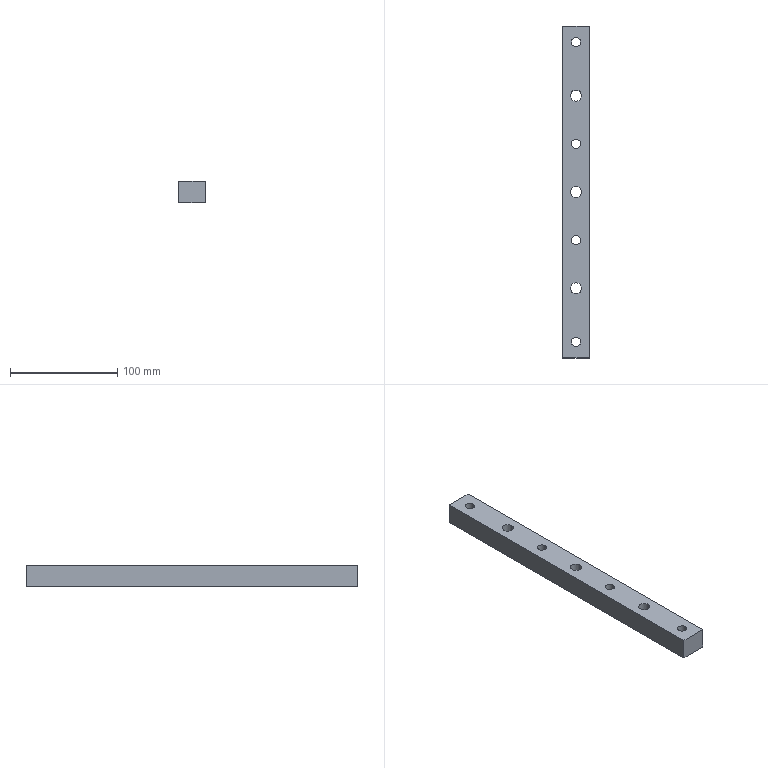Part | SolidWorks | features ICE 2, Extrusion 1, HoleWzd 1 | 1 solid | 32 faces | box 25 x 310 x 20 mm | volume 142225 mm3 | cylinder 22 | plane 10 | commonest cylinder face diameters 8.5 x8 13 x8 10.5 x6
STEP:
#1=CARTESIAN_POINT('',(5.25,90.,20.));
#2=VERTEX_POINT('',#1);
#3=CARTESIAN_POINT('',(-5.25,90.,20.));
#4=VERTEX_POINT('',#3);
#5=CARTESIAN_POINT('',(0.,90.,20.));
#6=DIRECTION('',(0.,0.,-1.));
#7=DIRECTION('',(-1.,0.,0.));
#8=AXIS2_PLACEMENT_3D('',#5,#6,#7);
#9=CIRCLE('',#8,5.25);
#10=EDGE_CURVE('',#2,#4,#9,.T.);
#11=ORIENTED_EDGE('',*,*,#10,.F.);
#12=CARTESIAN_POINT('',(5.25,90.,0.));
#13=VERTEX_POINT('',#12);
#14=CARTESIAN_POINT('',(5.25,90.,0.));
#15=DIRECTION('',(0.,0.,-1.));
#16=VECTOR('',#15,1000.);
#17=LINE('',#14,#16);
#18=EDGE_CURVE('',#2,#13,#17,.T.);
#19=ORIENTED_EDGE('',*,*,#18,.T.);
#20=CARTESIAN_POINT('',(-5.25,90.,0.));
#21=VERTEX_POINT('',#20);
#22=CARTESIAN_POINT('',(0.,90.,0.));
#23=DIRECTION('',(0.,0.,-1.));
#24=DIRECTION('',(-1.,0.,0.));
#25=AXIS2_PLACEMENT_3D('',#22,#23,#24);
#26=CIRCLE('',#25,5.25);
#27=EDGE_CURVE('',#13,#21,#26,.T.);
#28=ORIENTED_EDGE('',*,*,#27,.T.);
#29=CARTESIAN_POINT('',(-5.25,90.,0.));
#30=DIRECTION('',(0.,0.,-1.));
#31=VECTOR('',#30,1000.);
#32=LINE('',#29,#31);
#33=EDGE_CURVE('',#4,#21,#32,.T.);
#34=ORIENTED_EDGE('',*,*,#33,.F.);
#35=EDGE_LOOP('',(#11,#19,#28,#34));
#36=FACE_OUTER_BOUND('',#35,.T.);
#37=CARTESIAN_POINT('',(0.,90.,0.));
#38=DIRECTION('',(0.,0.,-1.));
#39=DIRECTION('',(-1.,0.,0.));
#40=AXIS2_PLACEMENT_3D('',#37,#38,#39);
#41=CYLINDRICAL_SURFACE('',#40,5.25);
#42=ADVANCED_FACE('',(#36),#41,.F.);
#43=CARTESIAN_POINT('',(5.25,0.,20.));
#44=VERTEX_POINT('',#43);
#45=CARTESIAN_POINT('',(-5.25,0.,20.));
#46=VERTEX_POINT('',#45);
#47=CARTESIAN_POINT('',(0.,0.,20.));
#48=DIRECTION('',(0.,0.,-1.));
#49=DIRECTION('',(-1.,0.,0.));
#50=AXIS2_PLACEMENT_3D('',#47,#48,#49);
#51=CIRCLE('',#50,5.25);
#52=EDGE_CURVE('',#44,#46,#51,.T.);
#53=ORIENTED_EDGE('',*,*,#52,.F.);
#54=CARTESIAN_POINT('',(5.25,0.,0.));
#55=VERTEX_POINT('',#54);
#56=CARTESIAN_POINT('',(5.25,0.,0.));
#57=DIRECTION('',(0.,0.,-1.));
#58=VECTOR('',#57,1000.);
#59=LINE('',#56,#58);
#60=EDGE_CURVE('',#44,#55,#59,.T.);
#61=ORIENTED_EDGE('',*,*,#60,.T.);
#62=CARTESIAN_POINT('',(-5.25,0.,0.));
#63=VERTEX_POINT('',#62);
#64=CARTESIAN_POINT('',(0.,0.,0.));
#65=DIRECTION('',(0.,0.,-1.));
#66=DIRECTION('',(-1.,0.,0.));
#67=AXIS2_PLACEMENT_3D('',#64,#65,#66);
#68=CIRCLE('',#67,5.25);
#69=EDGE_CURVE('',#55,#63,#68,.T.);
#70=ORIENTED_EDGE('',*,*,#69,.T.);
#71=CARTESIAN_POINT('',(-5.25,0.,0.));
#72=DIRECTION('',(0.,0.,-1.));
#73=VECTOR('',#72,1000.);
#74=LINE('',#71,#73);
#75=EDGE_CURVE('',#46,#63,#74,.T.);
#76=ORIENTED_EDGE('',*,*,#75,.F.);
#77=EDGE_LOOP('',(#53,#61,#70,#76));
#78=FACE_OUTER_BOUND('',#77,.T.);
#79=CARTESIAN_POINT('',(0.,0.,0.));
#80=DIRECTION('',(0.,0.,-1.));
#81=DIRECTION('',(-1.,0.,0.));
#82=AXIS2_PLACEMENT_3D('',#79,#80,#81);
#83=CYLINDRICAL_SURFACE('',#82,5.25);
#84=ADVANCED_FACE('',(#78),#83,.F.);
#85=CARTESIAN_POINT('',(5.25,-90.,20.));
#86=VERTEX_POINT('',#85);
#87=CARTESIAN_POINT('',(-5.25,-90.,20.));
#88=VERTEX_POINT('',#87);
#89=CARTESIAN_POINT('',(0.,-90.,20.));
#90=DIRECTION('',(0.,0.,-1.));
#91=DIRECTION('',(-1.,0.,0.));
#92=AXIS2_PLACEMENT_3D('',#89,#90,#91);
#93=CIRCLE('',#92,5.25);
#94=EDGE_CURVE('',#86,#88,#93,.T.);
#95=ORIENTED_EDGE('',*,*,#94,.F.);
#96=CARTESIAN_POINT('',(5.25,-90.,0.));
#97=VERTEX_POINT('',#96);
#98=CARTESIAN_POINT('',(5.25,-90.,0.));
#99=DIRECTION('',(0.,0.,-1.));
#100=VECTOR('',#99,1000.);
#101=LINE('',#98,#100);
#102=EDGE_CURVE('',#86,#97,#101,.T.);
#103=ORIENTED_EDGE('',*,*,#102,.T.);
#104=CARTESIAN_POINT('',(-5.25,-90.,0.));
#105=VERTEX_POINT('',#104);
#106=CARTESIAN_POINT('',(0.,-90.,0.));
#107=DIRECTION('',(0.,0.,-1.));
#108=DIRECTION('',(-1.,0.,0.));
#109=AXIS2_PLACEMENT_3D('',#106,#107,#108);
#110=CIRCLE('',#109,5.25);
#111=EDGE_CURVE('',#97,#105,#110,.T.);
#112=ORIENTED_EDGE('',*,*,#111,.T.);
#113=CARTESIAN_POINT('',(-5.25,-90.,0.));
#114=DIRECTION('',(0.,0.,-1.));
#115=VECTOR('',#114,1000.);
#116=LINE('',#113,#115);
#117=EDGE_CURVE('',#88,#105,#116,.T.);
#118=ORIENTED_EDGE('',*,*,#117,.F.);
#119=EDGE_LOOP('',(#95,#103,#112,#118));
#120=FACE_OUTER_BOUND('',#119,.T.);
#121=CARTESIAN_POINT('',(0.,-90.,0.));
#122=DIRECTION('',(0.,0.,-1.));
#123=DIRECTION('',(-1.,0.,0.));
#124=AXIS2_PLACEMENT_3D('',#121,#122,#123);
#125=CYLINDRICAL_SURFACE('',#124,5.25);
#126=ADVANCED_FACE('',(#120),#125,.F.);
#127=CARTESIAN_POINT('',(6.5,-140.,10.));
#128=VERTEX_POINT('',#127);
#129=CARTESIAN_POINT('',(-6.5,-140.,10.));
#130=VERTEX_POINT('',#129);
#131=CARTESIAN_POINT('',(0.,-140.,10.));
#132=DIRECTION('',(0.,0.,-1.));
#133=DIRECTION('',(-1.,0.,0.));
#134=AXIS2_PLACEMENT_3D('',#131,#132,#133);
#135=CIRCLE('',#134,6.5);
#136=EDGE_CURVE('',#128,#130,#135,.T.);
#137=ORIENTED_EDGE('',*,*,#136,.F.);
#138=CARTESIAN_POINT('',(6.5,-140.,0.));
#139=VERTEX_POINT('',#138);
#140=CARTESIAN_POINT('',(6.5,-140.,10.));
#141=DIRECTION('',(0.,0.,-1.));
#142=VECTOR('',#141,1000.);
#143=LINE('',#140,#142);
#144=EDGE_CURVE('',#128,#139,#143,.T.);
#145=ORIENTED_EDGE('',*,*,#144,.T.);
#146=CARTESIAN_POINT('',(-6.5,-140.,0.));
#147=VERTEX_POINT('',#146);
#148=CARTESIAN_POINT('',(0.,-140.,0.));
#149=DIRECTION('',(0.,0.,-1.));
#150=DIRECTION('',(-1.,0.,0.));
#151=AXIS2_PLACEMENT_3D('',#148,#149,#150);
#152=CIRCLE('',#151,6.5);
#153=EDGE_CURVE('',#139,#147,#152,.T.);
#154=ORIENTED_EDGE('',*,*,#153,.T.);
#155=CARTESIAN_POINT('',(-6.5,-140.,10.));
#156=DIRECTION('',(0.,0.,-1.));
#157=VECTOR('',#156,1000.);
#158=LINE('',#155,#157);
#159=EDGE_CURVE('',#130,#147,#158,.T.);
#160=ORIENTED_EDGE('',*,*,#159,.F.);
#161=EDGE_LOOP('',(#137,#145,#154,#160));
#162=FACE_OUTER_BOUND('',#161,.T.);
#163=CARTESIAN_POINT('',(0.,-140.,10.));
#164=DIRECTION('',(0.,0.,-1.));
#165=DIRECTION('',(-1.,0.,0.));
#166=AXIS2_PLACEMENT_3D('',#163,#164,#165);
#167=CYLINDRICAL_SURFACE('',#166,6.5);
#168=ADVANCED_FACE('',(#162),#167,.F.);
#169=CARTESIAN_POINT('',(6.5,-45.,10.));
#170=VERTEX_POINT('',#169);
#171=CARTESIAN_POINT('',(-6.5,-45.,10.));
#172=VERTEX_POINT('',#171);
#173=CARTESIAN_POINT('',(0.,-45.,10.));
#174=DIRECTION('',(0.,0.,-1.));
#175=DIRECTION('',(-1.,0.,0.));
#176=AXIS2_PLACEMENT_3D('',#173,#174,#175);
#177=CIRCLE('',#176,6.5);
#178=EDGE_CURVE('',#170,#172,#177,.T.);
#179=ORIENTED_EDGE('',*,*,#178,.F.);
#180=CARTESIAN_POINT('',(6.5,-45.,0.));
#181=VERTEX_POINT('',#180);
#182=CARTESIAN_POINT('',(6.5,-45.,10.));
#183=DIRECTION('',(0.,0.,-1.));
#184=VECTOR('',#183,1000.);
#185=LINE('',#182,#184);
#186=EDGE_CURVE('',#170,#181,#185,.T.);
#187=ORIENTED_EDGE('',*,*,#186,.T.);
#188=CARTESIAN_POINT('',(-6.5,-45.,0.));
#189=VERTEX_POINT('',#188);
#190=CARTESIAN_POINT('',(0.,-45.,0.));
#191=DIRECTION('',(0.,0.,-1.));
#192=DIRECTION('',(-1.,0.,0.));
#193=AXIS2_PLACEMENT_3D('',#190,#191,#192);
#194=CIRCLE('',#193,6.5);
#195=EDGE_CURVE('',#181,#189,#194,.T.);
#196=ORIENTED_EDGE('',*,*,#195,.T.);
#197=CARTESIAN_POINT('',(-6.5,-45.,10.));
#198=DIRECTION('',(0.,0.,-1.));
#199=VECTOR('',#198,1000.);
#200=LINE('',#197,#199);
#201=EDGE_CURVE('',#172,#189,#200,.T.);
#202=ORIENTED_EDGE('',*,*,#201,.F.);
#203=EDGE_LOOP('',(#179,#187,#196,#202));
#204=FACE_OUTER_BOUND('',#203,.T.);
#205=CARTESIAN_POINT('',(0.,-45.,10.));
#206=DIRECTION('',(0.,0.,-1.));
#207=DIRECTION('',(-1.,0.,0.));
#208=AXIS2_PLACEMENT_3D('',#205,#206,#207);
#209=CYLINDRICAL_SURFACE('',#208,6.5);
#210=ADVANCED_FACE('',(#204),#209,.F.);
#211=CARTESIAN_POINT('',(6.5,45.,10.));
#212=VERTEX_POINT('',#211);
#213=CARTESIAN_POINT('',(-6.5,45.,10.));
#214=VERTEX_POINT('',#213);
#215=CARTESIAN_POINT('',(0.,45.,10.));
#216=DIRECTION('',(0.,0.,-1.));
#217=DIRECTION('',(-1.,0.,0.));
#218=AXIS2_PLACEMENT_3D('',#215,#216,#217);
#219=CIRCLE('',#218,6.5);
#220=EDGE_CURVE('',#212,#214,#219,.T.);
#221=ORIENTED_EDGE('',*,*,#220,.F.);
#222=CARTESIAN_POINT('',(6.5,45.,0.));
#223=VERTEX_POINT('',#222);
#224=CARTESIAN_POINT('',(6.5,45.,10.));
#225=DIRECTION('',(0.,0.,-1.));
#226=VECTOR('',#225,1000.);
#227=LINE('',#224,#226);
#228=EDGE_CURVE('',#212,#223,#227,.T.);
#229=ORIENTED_EDGE('',*,*,#228,.T.);
#230=CARTESIAN_POINT('',(-6.5,45.,0.));
#231=VERTEX_POINT('',#230);
#232=CARTESIAN_POINT('',(0.,45.,0.));
#233=DIRECTION('',(0.,0.,-1.));
#234=DIRECTION('',(-1.,0.,0.));
#235=AXIS2_PLACEMENT_3D('',#232,#233,#234);
#236=CIRCLE('',#235,6.5);
#237=EDGE_CURVE('',#223,#231,#236,.T.);
#238=ORIENTED_EDGE('',*,*,#237,.T.);
#239=CARTESIAN_POINT('',(-6.5,45.,10.));
#240=DIRECTION('',(0.,0.,-1.));
#241=VECTOR('',#240,1000.);
#242=LINE('',#239,#241);
#243=EDGE_CURVE('',#214,#231,#242,.T.);
#244=ORIENTED_EDGE('',*,*,#243,.F.);
#245=EDGE_LOOP('',(#221,#229,#238,#244));
#246=FACE_OUTER_BOUND('',#245,.T.);
#247=CARTESIAN_POINT('',(0.,45.,10.));
#248=DIRECTION('',(0.,0.,-1.));
#249=DIRECTION('',(-1.,0.,0.));
#250=AXIS2_PLACEMENT_3D('',#247,#248,#249);
#251=CYLINDRICAL_SURFACE('',#250,6.5);
#252=ADVANCED_FACE('',(#246),#251,.F.);
#253=CARTESIAN_POINT('',(6.5,140.,10.));
#254=VERTEX_POINT('',#253);
#255=CARTESIAN_POINT('',(-6.5,140.,10.));
#256=VERTEX_POINT('',#255);
#257=CARTESIAN_POINT('',(0.,140.,10.));
#258=DIRECTION('',(0.,0.,-1.));
#259=DIRECTION('',(-1.,0.,0.));
#260=AXIS2_PLACEMENT_3D('',#257,#258,#259);
#261=CIRCLE('',#260,6.5);
#262=EDGE_CURVE('',#254,#256,#261,.T.);
#263=ORIENTED_EDGE('',*,*,#262,.F.);
#264=CARTESIAN_POINT('',(6.5,140.,0.));
#265=VERTEX_POINT('',#264);
#266=CARTESIAN_POINT('',(6.5,140.,10.));
#267=DIRECTION('',(0.,0.,-1.));
#268=VECTOR('',#267,1000.);
#269=LINE('',#266,#268);
#270=EDGE_CURVE('',#254,#265,#269,.T.);
#271=ORIENTED_EDGE('',*,*,#270,.T.);
#272=CARTESIAN_POINT('',(-6.5,140.,0.));
#273=VERTEX_POINT('',#272);
#274=CARTESIAN_POINT('',(0.,140.,0.));
#275=DIRECTION('',(0.,0.,-1.));
#276=DIRECTION('',(-1.,0.,0.));
#277=AXIS2_PLACEMENT_3D('',#274,#275,#276);
#278=CIRCLE('',#277,6.5);
#279=EDGE_CURVE('',#265,#273,#278,.T.);
#280=ORIENTED_EDGE('',*,*,#279,.T.);
#281=CARTESIAN_POINT('',(-6.5,140.,10.));
#282=DIRECTION('',(0.,0.,-1.));
#283=VECTOR('',#282,1000.);
#284=LINE('',#281,#283);
#285=EDGE_CURVE('',#256,#273,#284,.T.);
#286=ORIENTED_EDGE('',*,*,#285,.F.);
#287=EDGE_LOOP('',(#263,#271,#280,#286));
#288=FACE_OUTER_BOUND('',#287,.T.);
#289=CARTESIAN_POINT('',(0.,140.,10.));
#290=DIRECTION('',(0.,0.,-1.));
#291=DIRECTION('',(-1.,0.,0.));
#292=AXIS2_PLACEMENT_3D('',#289,#290,#291);
#293=CYLINDRICAL_SURFACE('',#292,6.5);
#294=ADVANCED_FACE('',(#288),#293,.F.);
#295=CARTESIAN_POINT('',(-4.25,140.,10.));
#296=VERTEX_POINT('',#295);
#297=CARTESIAN_POINT('',(4.25,140.,10.));
#298=VERTEX_POINT('',#297);
#299=CARTESIAN_POINT('',(0.,140.,10.));
#300=DIRECTION('',(0.,0.,1.));
#301=DIRECTION('',(-1.,0.,0.));
#302=AXIS2_PLACEMENT_3D('',#299,#300,#301);
#303=CIRCLE('',#302,4.25);
#304=EDGE_CURVE('',#296,#298,#303,.T.);
#305=ORIENTED_EDGE('',*,*,#304,.F.);
#306=CARTESIAN_POINT('',(-4.25,140.,20.));
#307=VERTEX_POINT('',#306);
#308=CARTESIAN_POINT('',(-4.25,140.,-10.));
#309=DIRECTION('',(0.,0.,1.));
#310=VECTOR('',#309,1000.);
#311=LINE('',#308,#310);
#312=EDGE_CURVE('',#296,#307,#311,.T.);
#313=ORIENTED_EDGE('',*,*,#312,.T.);
#314=CARTESIAN_POINT('',(4.25,140.,20.));
#315=VERTEX_POINT('',#314);
#316=CARTESIAN_POINT('',(0.,140.,20.));
#317=DIRECTION('',(0.,0.,1.));
#318=DIRECTION('',(1.,0.,0.));
#319=AXIS2_PLACEMENT_3D('',#316,#317,#318);
#320=CIRCLE('',#319,4.25);
#321=EDGE_CURVE('',#307,#315,#320,.T.);
#322=ORIENTED_EDGE('',*,*,#321,.T.);
#323=CARTESIAN_POINT('',(4.25,140.,-10.));
#324=DIRECTION('',(0.,0.,1.));
#325=VECTOR('',#324,1000.);
#326=LINE('',#323,#325);
#327=EDGE_CURVE('',#298,#315,#326,.T.);
#328=ORIENTED_EDGE('',*,*,#327,.F.);
#329=EDGE_LOOP('',(#305,#313,#322,#328));
#330=FACE_OUTER_BOUND('',#329,.T.);
#331=CARTESIAN_POINT('',(0.,140.,-10.));
#332=DIRECTION('',(0.,0.,1.));
#333=DIRECTION('',(1.,0.,0.));
#334=AXIS2_PLACEMENT_3D('',#331,#332,#333);
#335=CYLINDRICAL_SURFACE('',#334,4.25);
#336=ADVANCED_FACE('',(#330),#335,.F.);
#337=CARTESIAN_POINT('',(-4.25,45.,10.));
#338=VERTEX_POINT('',#337);
#339=CARTESIAN_POINT('',(4.25,45.,10.));
#340=VERTEX_POINT('',#339);
#341=CARTESIAN_POINT('',(0.,45.,10.));
#342=DIRECTION('',(0.,0.,1.));
#343=DIRECTION('',(-1.,0.,0.));
#344=AXIS2_PLACEMENT_3D('',#341,#342,#343);
#345=CIRCLE('',#344,4.25);
#346=EDGE_CURVE('',#338,#340,#345,.T.);
#347=ORIENTED_EDGE('',*,*,#346,.F.);
#348=CARTESIAN_POINT('',(-4.25,45.,20.));
#349=VERTEX_POINT('',#348);
#350=CARTESIAN_POINT('',(-4.25,45.,-10.));
#351=DIRECTION('',(0.,0.,1.));
#352=VECTOR('',#351,1000.);
#353=LINE('',#350,#352);
#354=EDGE_CURVE('',#338,#349,#353,.T.);
#355=ORIENTED_EDGE('',*,*,#354,.T.);
#356=CARTESIAN_POINT('',(4.25,45.,20.));
#357=VERTEX_POINT('',#356);
#358=CARTESIAN_POINT('',(0.,45.,20.));
#359=DIRECTION('',(0.,0.,1.));
#360=DIRECTION('',(1.,0.,0.));
#361=AXIS2_PLACEMENT_3D('',#358,#359,#360);
#362=CIRCLE('',#361,4.25);
#363=EDGE_CURVE('',#349,#357,#362,.T.);
#364=ORIENTED_EDGE('',*,*,#363,.T.);
#365=CARTESIAN_POINT('',(4.25,45.,-10.));
#366=DIRECTION('',(0.,0.,1.));
#367=VECTOR('',#366,1000.);
#368=LINE('',#365,#367);
#369=EDGE_CURVE('',#340,#357,#368,.T.);
#370=ORIENTED_EDGE('',*,*,#369,.F.);
#371=EDGE_LOOP('',(#347,#355,#364,#370));
#372=FACE_OUTER_BOUND('',#371,.T.);
#373=CARTESIAN_POINT('',(0.,45.,-10.));
#374=DIRECTION('',(0.,0.,1.));
#375=DIRECTION('',(1.,0.,0.));
#376=AXIS2_PLACEMENT_3D('',#373,#374,#375);
#377=CYLINDRICAL_SURFACE('',#376,4.25);
#378=ADVANCED_FACE('',(#372),#377,.F.);
#379=CARTESIAN_POINT('',(-4.25,-45.,10.));
#380=VERTEX_POINT('',#379);
#381=CARTESIAN_POINT('',(4.25,-45.,10.));
#382=VERTEX_POINT('',#381);
#383=CARTESIAN_POINT('',(0.,-45.,10.));
#384=DIRECTION('',(0.,0.,1.));
#385=DIRECTION('',(-1.,0.,0.));
#386=AXIS2_PLACEMENT_3D('',#383,#384,#385);
#387=CIRCLE('',#386,4.25);
#388=EDGE_CURVE('',#380,#382,#387,.T.);
#389=ORIENTED_EDGE('',*,*,#388,.F.);
#390=CARTESIAN_POINT('',(-4.25,-45.,20.));
#391=VERTEX_POINT('',#390);
#392=CARTESIAN_POINT('',(-4.25,-45.,-10.));
#393=DIRECTION('',(0.,0.,1.));
#394=VECTOR('',#393,1000.);
#395=LINE('',#392,#394);
#396=EDGE_CURVE('',#380,#391,#395,.T.);
#397=ORIENTED_EDGE('',*,*,#396,.T.);
#398=CARTESIAN_POINT('',(4.25,-45.,20.));
#399=VERTEX_POINT('',#398);
#400=CARTESIAN_POINT('',(0.,-45.,20.));
#401=DIRECTION('',(0.,0.,1.));
#402=DIRECTION('',(1.,0.,0.));
#403=AXIS2_PLACEMENT_3D('',#400,#401,#402);
#404=CIRCLE('',#403,4.25);
#405=EDGE_CURVE('',#391,#399,#404,.T.);
#406=ORIENTED_EDGE('',*,*,#405,.T.);
#407=CARTESIAN_POINT('',(4.25,-45.,-10.));
#408=DIRECTION('',(0.,0.,1.));
#409=VECTOR('',#408,1000.);
#410=LINE('',#407,#409);
#411=EDGE_CURVE('',#382,#399,#410,.T.);
#412=ORIENTED_EDGE('',*,*,#411,.F.);
#413=EDGE_LOOP('',(#389,#397,#406,#412));
#414=FACE_OUTER_BOUND('',#413,.T.);
#415=CARTESIAN_POINT('',(0.,-45.,-10.));
#416=DIRECTION('',(0.,0.,1.));
#417=DIRECTION('',(1.,0.,0.));
#418=AXIS2_PLACEMENT_3D('',#415,#416,#417);
#419=CYLINDRICAL_SURFACE('',#418,4.25);
#420=ADVANCED_FACE('',(#414),#419,.F.);
#421=CARTESIAN_POINT('',(-4.25,-140.,10.));
#422=VERTEX_POINT('',#421);
#423=CARTESIAN_POINT('',(4.25,-140.,10.));
#424=VERTEX_POINT('',#423);
#425=CARTESIAN_POINT('',(0.,-140.,10.));
#426=DIRECTION('',(0.,0.,1.));
#427=DIRECTION('',(-1.,0.,0.));
#428=AXIS2_PLACEMENT_3D('',#425,#426,#427);
#429=CIRCLE('',#428,4.25);
#430=EDGE_CURVE('',#422,#424,#429,.T.);
#431=ORIENTED_EDGE('',*,*,#430,.F.);
#432=CARTESIAN_POINT('',(-4.25,-140.,20.));
#433=VERTEX_POINT('',#432);
#434=CARTESIAN_POINT('',(-4.25,-140.,-10.));
#435=DIRECTION('',(0.,0.,1.));
#436=VECTOR('',#435,1000.);
#437=LINE('',#434,#436);
#438=EDGE_CURVE('',#422,#433,#437,.T.);
#439=ORIENTED_EDGE('',*,*,#438,.T.);
#440=CARTESIAN_POINT('',(4.25,-140.,20.));
#441=VERTEX_POINT('',#440);
#442=CARTESIAN_POINT('',(0.,-140.,20.));
#443=DIRECTION('',(0.,0.,1.));
#444=DIRECTION('',(1.,0.,0.));
#445=AXIS2_PLACEMENT_3D('',#442,#443,#444);
#446=CIRCLE('',#445,4.25);
#447=EDGE_CURVE('',#433,#441,#446,.T.);
#448=ORIENTED_EDGE('',*,*,#447,.T.);
#449=CARTESIAN_POINT('',(4.25,-140.,-10.));
#450=DIRECTION('',(0.,0.,1.));
#451=VECTOR('',#450,1000.);
#452=LINE('',#449,#451);
#453=EDGE_CURVE('',#424,#441,#452,.T.);
#454=ORIENTED_EDGE('',*,*,#453,.F.);
#455=EDGE_LOOP('',(#431,#439,#448,#454));
#456=FACE_OUTER_BOUND('',#455,.T.);
#457=CARTESIAN_POINT('',(0.,-140.,-10.));
#458=DIRECTION('',(0.,0.,1.));
#459=DIRECTION('',(1.,0.,0.));
#460=AXIS2_PLACEMENT_3D('',#457,#458,#459);
#461=CYLINDRICAL_SURFACE('',#460,4.25);
#462=ADVANCED_FACE('',(#456),#461,.F.);
#463=ORIENTED_EDGE('',*,*,#438,.F.);
#464=CARTESIAN_POINT('',(0.,-140.,10.));
#465=DIRECTION('',(0.,0.,1.));
#466=DIRECTION('',(-1.,0.,0.));
#467=AXIS2_PLACEMENT_3D('',#464,#465,#466);
#468=CIRCLE('',#467,4.25);
#469=EDGE_CURVE('',#424,#422,#468,.T.);
#470=ORIENTED_EDGE('',*,*,#469,.F.);
#471=ORIENTED_EDGE('',*,*,#453,.T.);
#472=CARTESIAN_POINT('',(0.,-140.,20.));
#473=DIRECTION('',(0.,0.,1.));
#474=DIRECTION('',(1.,0.,0.));
#475=AXIS2_PLACEMENT_3D('',#472,#473,#474);
#476=CIRCLE('',#475,4.25);
#477=EDGE_CURVE('',#441,#433,#476,.T.);
#478=ORIENTED_EDGE('',*,*,#477,.T.);
#479=EDGE_LOOP('',(#463,#470,#471,#478));
#480=FACE_OUTER_BOUND('',#479,.T.);
#481=CARTESIAN_POINT('',(0.,-140.,-10.));
#482=DIRECTION('',(0.,0.,1.));
#483=DIRECTION('',(1.,0.,0.));
#484=AXIS2_PLACEMENT_3D('',#481,#482,#483);
#485=CYLINDRICAL_SURFACE('',#484,4.25);
#486=ADVANCED_FACE('',(#480),#485,.F.);
#487=ORIENTED_EDGE('',*,*,#396,.F.);
#488=CARTESIAN_POINT('',(0.,-45.,10.));
#489=DIRECTION('',(0.,0.,1.));
#490=DIRECTION('',(-1.,0.,0.));
#491=AXIS2_PLACEMENT_3D('',#488,#489,#490);
#492=CIRCLE('',#491,4.25);
#493=EDGE_CURVE('',#382,#380,#492,.T.);
#494=ORIENTED_EDGE('',*,*,#493,.F.);
#495=ORIENTED_EDGE('',*,*,#411,.T.);
#496=CARTESIAN_POINT('',(0.,-45.,20.));
#497=DIRECTION('',(0.,0.,1.));
#498=DIRECTION('',(1.,0.,0.));
#499=AXIS2_PLACEMENT_3D('',#496,#497,#498);
#500=CIRCLE('',#499,4.25);
#501=EDGE_CURVE('',#399,#391,#500,.T.);
#502=ORIENTED_EDGE('',*,*,#501,.T.);
#503=EDGE_LOOP('',(#487,#494,#495,#502));
#504=FACE_OUTER_BOUND('',#503,.T.);
#505=CARTESIAN_POINT('',(0.,-45.,-10.));
#506=DIRECTION('',(0.,0.,1.));
#507=DIRECTION('',(1.,0.,0.));
#508=AXIS2_PLACEMENT_3D('',#505,#506,#507);
#509=CYLINDRICAL_SURFACE('',#508,4.25);
#510=ADVANCED_FACE('',(#504),#509,.F.);
#511=ORIENTED_EDGE('',*,*,#354,.F.);
#512=CARTESIAN_POINT('',(0.,45.,10.));
#513=DIRECTION('',(0.,0.,1.));
#514=DIRECTION('',(-1.,0.,0.));
#515=AXIS2_PLACEMENT_3D('',#512,#513,#514);
#516=CIRCLE('',#515,4.25);
#517=EDGE_CURVE('',#340,#338,#516,.T.);
#518=ORIENTED_EDGE('',*,*,#517,.F.);
#519=ORIENTED_EDGE('',*,*,#369,.T.);
#520=CARTESIAN_POINT('',(0.,45.,20.));
#521=DIRECTION('',(0.,0.,1.));
#522=DIRECTION('',(1.,0.,0.));
#523=AXIS2_PLACEMENT_3D('',#520,#521,#522);
#524=CIRCLE('',#523,4.25);
#525=EDGE_CURVE('',#357,#349,#524,.T.);
#526=ORIENTED_EDGE('',*,*,#525,.T.);
#527=EDGE_LOOP('',(#511,#518,#519,#526));
#528=FACE_OUTER_BOUND('',#527,.T.);
#529=CARTESIAN_POINT('',(0.,45.,-10.));
#530=DIRECTION('',(0.,0.,1.));
#531=DIRECTION('',(1.,0.,0.));
#532=AXIS2_PLACEMENT_3D('',#529,#530,#531);
#533=CYLINDRICAL_SURFACE('',#532,4.25);
#534=ADVANCED_FACE('',(#528),#533,.F.);
#535=ORIENTED_EDGE('',*,*,#312,.F.);
#536=CARTESIAN_POINT('',(0.,140.,10.));
#537=DIRECTION('',(0.,0.,1.));
#538=DIRECTION('',(-1.,0.,0.));
#539=AXIS2_PLACEMENT_3D('',#536,#537,#538);
#540=CIRCLE('',#539,4.25);
#541=EDGE_CURVE('',#298,#296,#540,.T.);
#542=ORIENTED_EDGE('',*,*,#541,.F.);
#543=ORIENTED_EDGE('',*,*,#327,.T.);
#544=CARTESIAN_POINT('',(0.,140.,20.));
#545=DIRECTION('',(0.,0.,1.));
#546=DIRECTION('',(1.,0.,0.));
#547=AXIS2_PLACEMENT_3D('',#544,#545,#546);
#548=CIRCLE('',#547,4.25);
#549=EDGE_CURVE('',#315,#307,#548,.T.);
#550=ORIENTED_EDGE('',*,*,#549,.T.);
#551=EDGE_LOOP('',(#535,#542,#543,#550));
#552=FACE_OUTER_BOUND('',#551,.T.);
#553=CARTESIAN_POINT('',(0.,140.,-10.));
#554=DIRECTION('',(0.,0.,1.));
#555=DIRECTION('',(1.,0.,0.));
#556=AXIS2_PLACEMENT_3D('',#553,#554,#555);
#557=CYLINDRICAL_SURFACE('',#556,4.25);
#558=ADVANCED_FACE('',(#552),#557,.F.);
#559=CARTESIAN_POINT('',(12.5,-155.,0.));
#560=VERTEX_POINT('',#559);
#561=CARTESIAN_POINT('',(12.5,155.,0.));
#562=VERTEX_POINT('',#561);
#563=CARTESIAN_POINT('',(12.5,-155.,0.));
#564=DIRECTION('',(0.,1.,0.));
#565=VECTOR('',#564,1000.);
#566=LINE('',#563,#565);
#567=EDGE_CURVE('',#560,#562,#566,.T.);
#568=ORIENTED_EDGE('',*,*,#567,.T.);
#569=CARTESIAN_POINT('',(12.5,155.,20.));
#570=VERTEX_POINT('',#569);
#571=CARTESIAN_POINT('',(12.5,155.,20.));
#572=DIRECTION('',(0.,0.,-1.));
#573=VECTOR('',#572,1000.);
#574=LINE('',#571,#573);
#575=EDGE_CURVE('',#570,#562,#574,.T.);
#576=ORIENTED_EDGE('',*,*,#575,.F.);
#577=CARTESIAN_POINT('',(12.5,-155.,20.));
#578=VERTEX_POINT('',#577);
#579=CARTESIAN_POINT('',(12.5,-155.,20.));
#580=DIRECTION('',(0.,1.,0.));
#581=VECTOR('',#580,1000.);
#582=LINE('',#579,#581);
#583=EDGE_CURVE('',#578,#570,#582,.T.);
#584=ORIENTED_EDGE('',*,*,#583,.F.);
#585=CARTESIAN_POINT('',(12.5,-155.,20.));
#586=DIRECTION('',(0.,0.,-1.));
#587=VECTOR('',#586,1000.);
#588=LINE('',#585,#587);
#589=EDGE_CURVE('',#578,#560,#588,.T.);
#590=ORIENTED_EDGE('',*,*,#589,.T.);
#591=EDGE_LOOP('',(#568,#576,#584,#590));
#592=FACE_OUTER_BOUND('',#591,.T.);
#593=CARTESIAN_POINT('',(12.5,-155.,20.));
#594=DIRECTION('',(-1.,0.,0.));
#595=DIRECTION('',(0.,0.,1.));
#596=AXIS2_PLACEMENT_3D('',#593,#594,#595);
#597=PLANE('',#596);
#598=ADVANCED_FACE('',(#592),#597,.F.);
#599=CARTESIAN_POINT('',(-12.5,155.,0.));
#600=VERTEX_POINT('',#599);
#601=CARTESIAN_POINT('',(-12.5,155.,0.));
#602=DIRECTION('',(-1.,0.,0.));
#603=VECTOR('',#602,1000.);
#604=LINE('',#601,#603);
#605=EDGE_CURVE('',#562,#600,#604,.T.);
#606=ORIENTED_EDGE('',*,*,#605,.T.);
#607=CARTESIAN_POINT('',(-12.5,155.,20.));
#608=VERTEX_POINT('',#607);
#609=CARTESIAN_POINT('',(-12.5,155.,20.));
#610=DIRECTION('',(0.,0.,-1.));
#611=VECTOR('',#610,1000.);
#612=LINE('',#609,#611);
#613=EDGE_CURVE('',#608,#600,#612,.T.);
#614=ORIENTED_EDGE('',*,*,#613,.F.);
#615=CARTESIAN_POINT('',(-12.5,155.,20.));
#616=DIRECTION('',(-1.,0.,0.));
#617=VECTOR('',#616,1000.);
#618=LINE('',#615,#617);
#619=EDGE_CURVE('',#570,#608,#618,.T.);
#620=ORIENTED_EDGE('',*,*,#619,.F.);
#621=ORIENTED_EDGE('',*,*,#575,.T.);
#622=EDGE_LOOP('',(#606,#614,#620,#621));
#623=FACE_OUTER_BOUND('',#622,.T.);
#624=CARTESIAN_POINT('',(-12.5,155.,20.));
#625=DIRECTION('',(0.,-1.,0.));
#626=DIRECTION('',(0.,0.,-1.));
#627=AXIS2_PLACEMENT_3D('',#624,#625,#626);
#628=PLANE('',#627);
#629=ADVANCED_FACE('',(#623),#628,.F.);
#630=CARTESIAN_POINT('',(-12.5,-155.,0.));
#631=VERTEX_POINT('',#630);
#632=CARTESIAN_POINT('',(-12.5,-155.,0.));
#633=DIRECTION('',(0.,-1.,0.));
#634=VECTOR('',#633,1000.);
#635=LINE('',#632,#634);
#636=EDGE_CURVE('',#600,#631,#635,.T.);
#637=ORIENTED_EDGE('',*,*,#636,.T.);
#638=CARTESIAN_POINT('',(-12.5,-155.,20.));
#639=VERTEX_POINT('',#638);
#640=CARTESIAN_POINT('',(-12.5,-155.,20.));
#641=DIRECTION('',(0.,0.,-1.));
#642=VECTOR('',#641,1000.);
#643=LINE('',#640,#642);
#644=EDGE_CURVE('',#639,#631,#643,.T.);
#645=ORIENTED_EDGE('',*,*,#644,.F.);
#646=CARTESIAN_POINT('',(-12.5,-155.,20.));
#647=DIRECTION('',(0.,-1.,0.));
#648=VECTOR('',#647,1000.);
#649=LINE('',#646,#648);
#650=EDGE_CURVE('',#608,#639,#649,.T.);
#651=ORIENTED_EDGE('',*,*,#650,.F.);
#652=ORIENTED_EDGE('',*,*,#613,.T.);
#653=EDGE_LOOP('',(#637,#645,#651,#652));
#654=FACE_OUTER_BOUND('',#653,.T.);
#655=CARTESIAN_POINT('',(-12.5,-155.,20.));
#656=DIRECTION('',(1.,0.,0.));
#657=DIRECTION('',(0.,0.,-1.));
#658=AXIS2_PLACEMENT_3D('',#655,#656,#657);
#659=PLANE('',#658);
#660=ADVANCED_FACE('',(#654),#659,.F.);
#661=CARTESIAN_POINT('',(-12.5,-155.,0.));
#662=DIRECTION('',(1.,0.,0.));
#663=VECTOR('',#662,1000.);
#664=LINE('',#661,#663);
#665=EDGE_CURVE('',#631,#560,#664,.T.);
#666=ORIENTED_EDGE('',*,*,#665,.T.);
#667=ORIENTED_EDGE('',*,*,#589,.F.);
#668=CARTESIAN_POINT('',(-12.5,-155.,20.));
#669=DIRECTION('',(1.,0.,0.));
#670=VECTOR('',#669,1000.);
#671=LINE('',#668,#670);
#672=EDGE_CURVE('',#639,#578,#671,.T.);
#673=ORIENTED_EDGE('',*,*,#672,.F.);
#674=ORIENTED_EDGE('',*,*,#644,.T.);
#675=EDGE_LOOP('',(#666,#667,#673,#674));
#676=FACE_OUTER_BOUND('',#675,.T.);
#677=CARTESIAN_POINT('',(-12.5,-155.,20.));
#678=DIRECTION('',(0.,1.,0.));
#679=DIRECTION('',(0.,0.,1.));
#680=AXIS2_PLACEMENT_3D('',#677,#678,#679);
#681=PLANE('',#680);
#682=ADVANCED_FACE('',(#676),#681,.F.);
#683=CARTESIAN_POINT('',(0.,90.,20.));
#684=DIRECTION('',(0.,0.,-1.));
#685=DIRECTION('',(-1.,0.,0.));
#686=AXIS2_PLACEMENT_3D('',#683,#684,#685);
#687=CIRCLE('',#686,5.25);
#688=EDGE_CURVE('',#4,#2,#687,.T.);
#689=ORIENTED_EDGE('',*,*,#688,.T.);
#690=ORIENTED_EDGE('',*,*,#10,.T.);
#691=EDGE_LOOP('',(#689,#690));
#692=FACE_BOUND('',#691,.T.);
#693=CARTESIAN_POINT('',(0.,0.,20.));
#694=DIRECTION('',(0.,0.,-1.));
#695=DIRECTION('',(-1.,0.,0.));
#696=AXIS2_PLACEMENT_3D('',#693,#694,#695);
#697=CIRCLE('',#696,5.25);
#698=EDGE_CURVE('',#46,#44,#697,.T.);
#699=ORIENTED_EDGE('',*,*,#698,.T.);
#700=ORIENTED_EDGE('',*,*,#52,.T.);
#701=EDGE_LOOP('',(#699,#700));
#702=FACE_BOUND('',#701,.T.);
#703=CARTESIAN_POINT('',(0.,-90.,20.));
#704=DIRECTION('',(0.,0.,-1.));
#705=DIRECTION('',(-1.,0.,0.));
#706=AXIS2_PLACEMENT_3D('',#703,#704,#705);
#707=CIRCLE('',#706,5.25);
#708=EDGE_CURVE('',#88,#86,#707,.T.);
#709=ORIENTED_EDGE('',*,*,#708,.T.);
#710=ORIENTED_EDGE('',*,*,#94,.T.);
#711=EDGE_LOOP('',(#709,#710));
#712=FACE_BOUND('',#711,.T.);
#713=ORIENTED_EDGE('',*,*,#477,.F.);
#714=ORIENTED_EDGE('',*,*,#447,.F.);
#715=EDGE_LOOP('',(#713,#714));
#716=FACE_BOUND('',#715,.T.);
#717=ORIENTED_EDGE('',*,*,#501,.F.);
#718=ORIENTED_EDGE('',*,*,#405,.F.);
#719=EDGE_LOOP('',(#717,#718));
#720=FACE_BOUND('',#719,.T.);
#721=ORIENTED_EDGE('',*,*,#525,.F.);
#722=ORIENTED_EDGE('',*,*,#363,.F.);
#723=EDGE_LOOP('',(#721,#722));
#724=FACE_BOUND('',#723,.T.);
#725=ORIENTED_EDGE('',*,*,#549,.F.);
#726=ORIENTED_EDGE('',*,*,#321,.F.);
#727=EDGE_LOOP('',(#725,#726));
#728=FACE_BOUND('',#727,.T.);
#729=ORIENTED_EDGE('',*,*,#583,.T.);
#730=ORIENTED_EDGE('',*,*,#619,.T.);
#731=ORIENTED_EDGE('',*,*,#650,.T.);
#732=ORIENTED_EDGE('',*,*,#672,.T.);
#733=EDGE_LOOP('',(#729,#730,#731,#732));
#734=FACE_OUTER_BOUND('',#733,.T.);
#735=CARTESIAN_POINT('',(0.,0.,20.));
#736=DIRECTION('',(0.,0.,-1.));
#737=DIRECTION('',(-1.,0.,0.));
#738=AXIS2_PLACEMENT_3D('',#735,#736,#737);
#739=PLANE('',#738);
#740=ADVANCED_FACE('',(#692,#702,#712,#716,#720,#724,#728,#734),#739,.F.);
#741=CARTESIAN_POINT('',(0.,90.,0.));
#742=DIRECTION('',(0.,0.,-1.));
#743=DIRECTION('',(-1.,0.,0.));
#744=AXIS2_PLACEMENT_3D('',#741,#742,#743);
#745=CIRCLE('',#744,5.25);
#746=EDGE_CURVE('',#21,#13,#745,.T.);
#747=ORIENTED_EDGE('',*,*,#746,.F.);
#748=ORIENTED_EDGE('',*,*,#27,.F.);
#749=EDGE_LOOP('',(#747,#748));
#750=FACE_BOUND('',#749,.T.);
#751=CARTESIAN_POINT('',(0.,0.,0.));
#752=DIRECTION('',(0.,0.,-1.));
#753=DIRECTION('',(-1.,0.,0.));
#754=AXIS2_PLACEMENT_3D('',#751,#752,#753);
#755=CIRCLE('',#754,5.25);
#756=EDGE_CURVE('',#63,#55,#755,.T.);
#757=ORIENTED_EDGE('',*,*,#756,.F.);
#758=ORIENTED_EDGE('',*,*,#69,.F.);
#759=EDGE_LOOP('',(#757,#758));
#760=FACE_BOUND('',#759,.T.);
#761=CARTESIAN_POINT('',(0.,-90.,0.));
#762=DIRECTION('',(0.,0.,-1.));
#763=DIRECTION('',(-1.,0.,0.));
#764=AXIS2_PLACEMENT_3D('',#761,#762,#763);
#765=CIRCLE('',#764,5.25);
#766=EDGE_CURVE('',#105,#97,#765,.T.);
#767=ORIENTED_EDGE('',*,*,#766,.F.);
#768=ORIENTED_EDGE('',*,*,#111,.F.);
#769=EDGE_LOOP('',(#767,#768));
#770=FACE_BOUND('',#769,.T.);
#771=CARTESIAN_POINT('',(0.,-140.,0.));
#772=DIRECTION('',(0.,0.,-1.));
#773=DIRECTION('',(-1.,0.,0.));
#774=AXIS2_PLACEMENT_3D('',#771,#772,#773);
#775=CIRCLE('',#774,6.5);
#776=EDGE_CURVE('',#147,#139,#775,.T.);
#777=ORIENTED_EDGE('',*,*,#776,.F.);
#778=ORIENTED_EDGE('',*,*,#153,.F.);
#779=EDGE_LOOP('',(#777,#778));
#780=FACE_BOUND('',#779,.T.);
#781=CARTESIAN_POINT('',(0.,-45.,0.));
#782=DIRECTION('',(0.,0.,-1.));
#783=DIRECTION('',(-1.,0.,0.));
#784=AXIS2_PLACEMENT_3D('',#781,#782,#783);
#785=CIRCLE('',#784,6.5);
#786=EDGE_CURVE('',#189,#181,#785,.T.);
#787=ORIENTED_EDGE('',*,*,#786,.F.);
#788=ORIENTED_EDGE('',*,*,#195,.F.);
#789=EDGE_LOOP('',(#787,#788));
#790=FACE_BOUND('',#789,.T.);
#791=CARTESIAN_POINT('',(0.,45.,0.));
#792=DIRECTION('',(0.,0.,-1.));
#793=DIRECTION('',(-1.,0.,0.));
#794=AXIS2_PLACEMENT_3D('',#791,#792,#793);
#795=CIRCLE('',#794,6.5);
#796=EDGE_CURVE('',#231,#223,#795,.T.);
#797=ORIENTED_EDGE('',*,*,#796,.F.);
#798=ORIENTED_EDGE('',*,*,#237,.F.);
#799=EDGE_LOOP('',(#797,#798));
#800=FACE_BOUND('',#799,.T.);
#801=CARTESIAN_POINT('',(0.,140.,0.));
#802=DIRECTION('',(0.,0.,-1.));
#803=DIRECTION('',(-1.,0.,0.));
#804=AXIS2_PLACEMENT_3D('',#801,#802,#803);
#805=CIRCLE('',#804,6.5);
#806=EDGE_CURVE('',#273,#265,#805,.T.);
#807=ORIENTED_EDGE('',*,*,#806,.F.);
#808=ORIENTED_EDGE('',*,*,#279,.F.);
#809=EDGE_LOOP('',(#807,#808));
#810=FACE_BOUND('',#809,.T.);
#811=ORIENTED_EDGE('',*,*,#567,.F.);
#812=ORIENTED_EDGE('',*,*,#665,.F.);
#813=ORIENTED_EDGE('',*,*,#636,.F.);
#814=ORIENTED_EDGE('',*,*,#605,.F.);
#815=EDGE_LOOP('',(#811,#812,#813,#814));
#816=FACE_OUTER_BOUND('',#815,.T.);
#817=CARTESIAN_POINT('',(0.,0.,0.));
#818=DIRECTION('',(0.,0.,-1.));
#819=DIRECTION('',(-1.,0.,0.));
#820=AXIS2_PLACEMENT_3D('',#817,#818,#819);
#821=PLANE('',#820);
#822=ADVANCED_FACE('',(#750,#760,#770,#780,#790,#800,#810,#816),#821,.T.);
#823=CARTESIAN_POINT('',(0.,140.,10.));
#824=DIRECTION('',(0.,0.,-1.));
#825=DIRECTION('',(-1.,0.,0.));
#826=AXIS2_PLACEMENT_3D('',#823,#824,#825);
#827=CIRCLE('',#826,6.5);
#828=EDGE_CURVE('',#256,#254,#827,.T.);
#829=ORIENTED_EDGE('',*,*,#828,.T.);
#830=ORIENTED_EDGE('',*,*,#262,.T.);
#831=EDGE_LOOP('',(#829,#830));
#832=FACE_OUTER_BOUND('',#831,.T.);
#833=ORIENTED_EDGE('',*,*,#541,.T.);
#834=ORIENTED_EDGE('',*,*,#304,.T.);
#835=EDGE_LOOP('',(#833,#834));
#836=FACE_BOUND('',#835,.T.);
#837=CARTESIAN_POINT('',(0.,140.,10.));
#838=DIRECTION('',(0.,0.,-1.));
#839=DIRECTION('',(-1.,0.,0.));
#840=AXIS2_PLACEMENT_3D('',#837,#838,#839);
#841=PLANE('',#840);
#842=ADVANCED_FACE('',(#832,#836),#841,.T.);
#843=ORIENTED_EDGE('',*,*,#270,.F.);
#844=ORIENTED_EDGE('',*,*,#828,.F.);
#845=ORIENTED_EDGE('',*,*,#285,.T.);
#846=ORIENTED_EDGE('',*,*,#806,.T.);
#847=EDGE_LOOP('',(#843,#844,#845,#846));
#848=FACE_OUTER_BOUND('',#847,.T.);
#849=CARTESIAN_POINT('',(0.,140.,10.));
#850=DIRECTION('',(0.,0.,-1.));
#851=DIRECTION('',(-1.,0.,0.));
#852=AXIS2_PLACEMENT_3D('',#849,#850,#851);
#853=CYLINDRICAL_SURFACE('',#852,6.5);
#854=ADVANCED_FACE('',(#848),#853,.F.);
#855=CARTESIAN_POINT('',(0.,45.,10.));
#856=DIRECTION('',(0.,0.,-1.));
#857=DIRECTION('',(-1.,0.,0.));
#858=AXIS2_PLACEMENT_3D('',#855,#856,#857);
#859=CIRCLE('',#858,6.5);
#860=EDGE_CURVE('',#214,#212,#859,.T.);
#861=ORIENTED_EDGE('',*,*,#860,.T.);
#862=ORIENTED_EDGE('',*,*,#220,.T.);
#863=EDGE_LOOP('',(#861,#862));
#864=FACE_OUTER_BOUND('',#863,.T.);
#865=ORIENTED_EDGE('',*,*,#517,.T.);
#866=ORIENTED_EDGE('',*,*,#346,.T.);
#867=EDGE_LOOP('',(#865,#866));
#868=FACE_BOUND('',#867,.T.);
#869=CARTESIAN_POINT('',(0.,45.,10.));
#870=DIRECTION('',(0.,0.,-1.));
#871=DIRECTION('',(-1.,0.,0.));
#872=AXIS2_PLACEMENT_3D('',#869,#870,#871);
#873=PLANE('',#872);
#874=ADVANCED_FACE('',(#864,#868),#873,.T.);
#875=ORIENTED_EDGE('',*,*,#228,.F.);
#876=ORIENTED_EDGE('',*,*,#860,.F.);
#877=ORIENTED_EDGE('',*,*,#243,.T.);
#878=ORIENTED_EDGE('',*,*,#796,.T.);
#879=EDGE_LOOP('',(#875,#876,#877,#878));
#880=FACE_OUTER_BOUND('',#879,.T.);
#881=CARTESIAN_POINT('',(0.,45.,10.));
#882=DIRECTION('',(0.,0.,-1.));
#883=DIRECTION('',(-1.,0.,0.));
#884=AXIS2_PLACEMENT_3D('',#881,#882,#883);
#885=CYLINDRICAL_SURFACE('',#884,6.5);
#886=ADVANCED_FACE('',(#880),#885,.F.);
#887=CARTESIAN_POINT('',(0.,-45.,10.));
#888=DIRECTION('',(0.,0.,-1.));
#889=DIRECTION('',(-1.,0.,0.));
#890=AXIS2_PLACEMENT_3D('',#887,#888,#889);
#891=CIRCLE('',#890,6.5);
#892=EDGE_CURVE('',#172,#170,#891,.T.);
#893=ORIENTED_EDGE('',*,*,#892,.T.);
#894=ORIENTED_EDGE('',*,*,#178,.T.);
#895=EDGE_LOOP('',(#893,#894));
#896=FACE_OUTER_BOUND('',#895,.T.);
#897=ORIENTED_EDGE('',*,*,#493,.T.);
#898=ORIENTED_EDGE('',*,*,#388,.T.);
#899=EDGE_LOOP('',(#897,#898));
#900=FACE_BOUND('',#899,.T.);
#901=CARTESIAN_POINT('',(0.,-45.,10.));
#902=DIRECTION('',(0.,0.,-1.));
#903=DIRECTION('',(-1.,0.,0.));
#904=AXIS2_PLACEMENT_3D('',#901,#902,#903);
#905=PLANE('',#904);
#906=ADVANCED_FACE('',(#896,#900),#905,.T.);
#907=ORIENTED_EDGE('',*,*,#186,.F.);
#908=ORIENTED_EDGE('',*,*,#892,.F.);
#909=ORIENTED_EDGE('',*,*,#201,.T.);
#910=ORIENTED_EDGE('',*,*,#786,.T.);
#911=EDGE_LOOP('',(#907,#908,#909,#910));
#912=FACE_OUTER_BOUND('',#911,.T.);
#913=CARTESIAN_POINT('',(0.,-45.,10.));
#914=DIRECTION('',(0.,0.,-1.));
#915=DIRECTION('',(-1.,0.,0.));
#916=AXIS2_PLACEMENT_3D('',#913,#914,#915);
#917=CYLINDRICAL_SURFACE('',#916,6.5);
#918=ADVANCED_FACE('',(#912),#917,.F.);
#919=CARTESIAN_POINT('',(0.,-140.,10.));
#920=DIRECTION('',(0.,0.,-1.));
#921=DIRECTION('',(-1.,0.,0.));
#922=AXIS2_PLACEMENT_3D('',#919,#920,#921);
#923=CIRCLE('',#922,6.5);
#924=EDGE_CURVE('',#130,#128,#923,.T.);
#925=ORIENTED_EDGE('',*,*,#924,.T.);
#926=ORIENTED_EDGE('',*,*,#136,.T.);
#927=EDGE_LOOP('',(#925,#926));
#928=FACE_OUTER_BOUND('',#927,.T.);
#929=ORIENTED_EDGE('',*,*,#469,.T.);
#930=ORIENTED_EDGE('',*,*,#430,.T.);
#931=EDGE_LOOP('',(#929,#930));
#932=FACE_BOUND('',#931,.T.);
#933=CARTESIAN_POINT('',(0.,-140.,10.));
#934=DIRECTION('',(0.,0.,-1.));
#935=DIRECTION('',(-1.,0.,0.));
#936=AXIS2_PLACEMENT_3D('',#933,#934,#935);
#937=PLANE('',#936);
#938=ADVANCED_FACE('',(#928,#932),#937,.T.);
#939=ORIENTED_EDGE('',*,*,#144,.F.);
#940=ORIENTED_EDGE('',*,*,#924,.F.);
#941=ORIENTED_EDGE('',*,*,#159,.T.);
#942=ORIENTED_EDGE('',*,*,#776,.T.);
#943=EDGE_LOOP('',(#939,#940,#941,#942));
#944=FACE_OUTER_BOUND('',#943,.T.);
#945=CARTESIAN_POINT('',(0.,-140.,10.));
#946=DIRECTION('',(0.,0.,-1.));
#947=DIRECTION('',(-1.,0.,0.));
#948=AXIS2_PLACEMENT_3D('',#945,#946,#947);
#949=CYLINDRICAL_SURFACE('',#948,6.5);
#950=ADVANCED_FACE('',(#944),#949,.F.);
#951=ORIENTED_EDGE('',*,*,#102,.F.);
#952=ORIENTED_EDGE('',*,*,#708,.F.);
#953=ORIENTED_EDGE('',*,*,#117,.T.);
#954=ORIENTED_EDGE('',*,*,#766,.T.);
#955=EDGE_LOOP('',(#951,#952,#953,#954));
#956=FACE_OUTER_BOUND('',#955,.T.);
#957=CARTESIAN_POINT('',(0.,-90.,0.));
#958=DIRECTION('',(0.,0.,-1.));
#959=DIRECTION('',(-1.,0.,0.));
#960=AXIS2_PLACEMENT_3D('',#957,#958,#959);
#961=CYLINDRICAL_SURFACE('',#960,5.25);
#962=ADVANCED_FACE('',(#956),#961,.F.);
#963=ORIENTED_EDGE('',*,*,#60,.F.);
#964=ORIENTED_EDGE('',*,*,#698,.F.);
#965=ORIENTED_EDGE('',*,*,#75,.T.);
#966=ORIENTED_EDGE('',*,*,#756,.T.);
#967=EDGE_LOOP('',(#963,#964,#965,#966));
#968=FACE_OUTER_BOUND('',#967,.T.);
#969=CARTESIAN_POINT('',(0.,0.,0.));
#970=DIRECTION('',(0.,0.,-1.));
#971=DIRECTION('',(-1.,0.,0.));
#972=AXIS2_PLACEMENT_3D('',#969,#970,#971);
#973=CYLINDRICAL_SURFACE('',#972,5.25);
#974=ADVANCED_FACE('',(#968),#973,.F.);
#975=ORIENTED_EDGE('',*,*,#18,.F.);
#976=ORIENTED_EDGE('',*,*,#688,.F.);
#977=ORIENTED_EDGE('',*,*,#33,.T.);
#978=ORIENTED_EDGE('',*,*,#746,.T.);
#979=EDGE_LOOP('',(#975,#976,#977,#978));
#980=FACE_OUTER_BOUND('',#979,.T.);
#981=CARTESIAN_POINT('',(0.,90.,0.));
#982=DIRECTION('',(0.,0.,-1.));
#983=DIRECTION('',(-1.,0.,0.));
#984=AXIS2_PLACEMENT_3D('',#981,#982,#983);
#985=CYLINDRICAL_SURFACE('',#984,5.25);
#986=ADVANCED_FACE('',(#980),#985,.F.);
#987=CLOSED_SHELL('',(#42,#84,#126,#168,#210,#252,#294,#336,#378,#420,#462,#486,#510,#534,#558,#598,#629,#660,#682,#740,#822,#842,#854,#874,#886,#906,#918,#938,#950,#962,#974,#986));
#988=MANIFOLD_SOLID_BREP('',#987);
#989=CARTESIAN_POINT('',(0.,0.,0.));
#990=DIRECTION('',(0.,0.,1.));
#991=DIRECTION('',(1.,0.,0.));
#992=AXIS2_PLACEMENT_3D('',#989,#990,#991);
#993=(LENGTH_UNIT()NAMED_UNIT(*)SI_UNIT(.MILLI.,.METRE.));
#994=UNCERTAINTY_MEASURE_WITH_UNIT(LENGTH_MEASURE(0.00001),#993,'','');
#995=(NAMED_UNIT(*)PLANE_ANGLE_UNIT()SI_UNIT($,.RADIAN.));
#996=(NAMED_UNIT(*)SI_UNIT($,.STERADIAN.)SOLID_ANGLE_UNIT());
#997=(GEOMETRIC_REPRESENTATION_CONTEXT(3)GLOBAL_UNCERTAINTY_ASSIGNED_CONTEXT((#994))GLOBAL_UNIT_ASSIGNED_CONTEXT((#993,#995,#996))REPRESENTATION_CONTEXT('',''));
#998=ADVANCED_BREP_SHAPE_REPRESENTATION('',(#988,#992),#997);